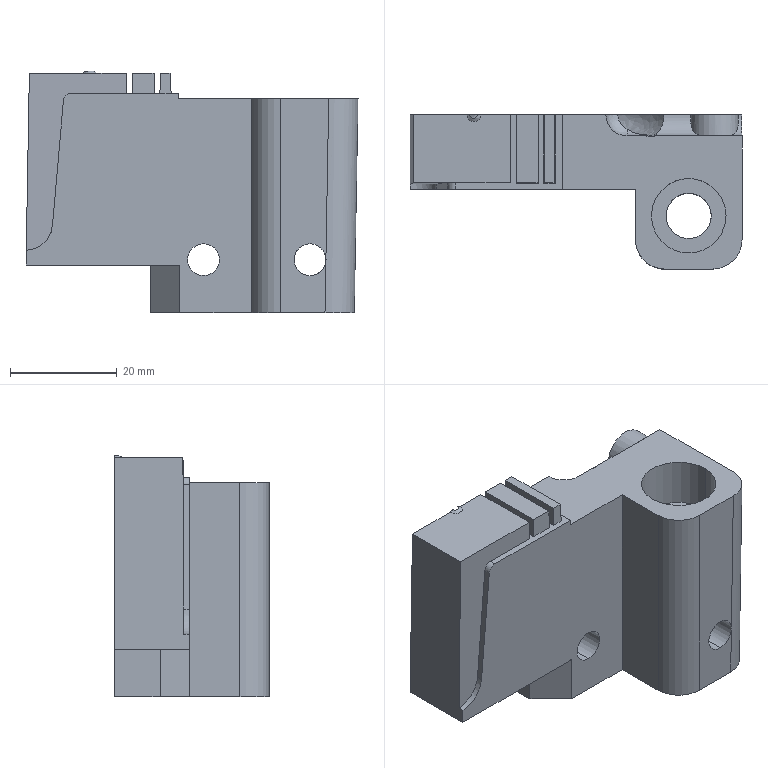Part | Creo | 1 solid | 185 faces | box 62.341 x 29 x 45.424 mm | volume 39530 mm3 | other 107 | plane 53 | cylinder 19 | sphere 3 | spline 2 | cone 1 | commonest cylinder face diameters 6 x6 8 x3 8.5 x2 11 x2 14 x2 3.012 x1